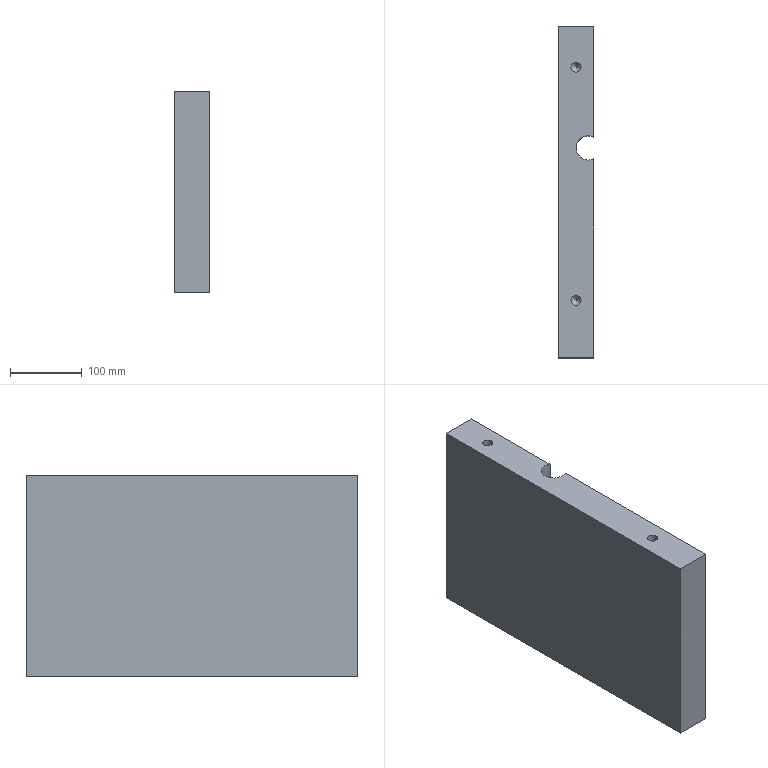Part | NX | features 29 2 | 1 solid | 16 faces | box 50 x 462.5 x 280.5 mm | volume 6261303 mm3 | plane 7 | cylinder 5 | cone 4 | commonest cylinder face diameters 14.1 x4 34 x1
STEP:
#1=CARTESIAN_POINT('',(867.05,-202.5,-493.5));
#2=VERTEX_POINT('',#1);
#3=CARTESIAN_POINT('',(860.,-202.5,-493.5));
#4=DIRECTION('',(0.,0.,1.));
#5=DIRECTION('',(1.,0.,0.));
#6=AXIS2_PLACEMENT_3D('',#3,#4,#5);
#7=CIRCLE('',#6,7.05);
#8=EDGE_CURVE('',#2,#2,#7,.T.);
#9=ORIENTED_EDGE('',*,*,#8,.T.);
#10=EDGE_LOOP('',(#9));
#11=FACE_BOUND('',#10,.T.);
#12=CARTESIAN_POINT('',(885.,-300.,-493.5));
#13=VERTEX_POINT('',#12);
#14=CARTESIAN_POINT('',(885.,-145.,-493.5));
#15=VERTEX_POINT('',#14);
#16=CARTESIAN_POINT('',(885.,193.,-493.5));
#17=DIRECTION('',(0.,1.,0.));
#18=VECTOR('',#17,1000.);
#19=LINE('',#16,#18);
#20=EDGE_CURVE('',#13,#15,#19,.T.);
#21=ORIENTED_EDGE('',*,*,#20,.F.);
#22=CARTESIAN_POINT('',(885.,-330.,-493.5));
#23=VERTEX_POINT('',#22);
#24=CARTESIAN_POINT('',(877.,-315.,-493.5));
#25=DIRECTION('',(0.,0.,1.));
#26=DIRECTION('',(-1.,0.,0.));
#27=AXIS2_PLACEMENT_3D('',#24,#25,#26);
#28=CIRCLE('',#27,17.);
#29=EDGE_CURVE('',#13,#23,#28,.T.);
#30=ORIENTED_EDGE('',*,*,#29,.T.);
#31=CARTESIAN_POINT('',(885.,-607.5,-493.5));
#32=VERTEX_POINT('',#31);
#33=CARTESIAN_POINT('',(885.,193.,-493.5));
#34=DIRECTION('',(0.,1.,0.));
#35=VECTOR('',#34,1000.);
#36=LINE('',#33,#35);
#37=EDGE_CURVE('',#32,#23,#36,.T.);
#38=ORIENTED_EDGE('',*,*,#37,.F.);
#39=CARTESIAN_POINT('',(835.,-607.5,-493.5));
#40=VERTEX_POINT('',#39);
#41=CARTESIAN_POINT('',(1635.,-607.5,-493.5));
#42=DIRECTION('',(-1.,0.,0.));
#43=VECTOR('',#42,1000.);
#44=LINE('',#41,#43);
#45=EDGE_CURVE('',#32,#40,#44,.T.);
#46=ORIENTED_EDGE('',*,*,#45,.T.);
#47=CARTESIAN_POINT('',(835.,-145.,-493.5));
#48=VERTEX_POINT('',#47);
#49=CARTESIAN_POINT('',(835.,193.,-493.5));
#50=DIRECTION('',(0.,-1.,0.));
#51=VECTOR('',#50,1000.);
#52=LINE('',#49,#51);
#53=EDGE_CURVE('',#48,#40,#52,.T.);
#54=ORIENTED_EDGE('',*,*,#53,.F.);
#55=CARTESIAN_POINT('',(1635.,-145.,-493.5));
#56=DIRECTION('',(-1.,0.,0.));
#57=VECTOR('',#56,1000.);
#58=LINE('',#55,#57);
#59=EDGE_CURVE('',#15,#48,#58,.T.);
#60=ORIENTED_EDGE('',*,*,#59,.F.);
#61=EDGE_LOOP('',(#21,#30,#38,#46,#54,#60));
#62=FACE_BOUND('',#61,.T.);
#63=CARTESIAN_POINT('',(867.05,-527.5,-493.5));
#64=VERTEX_POINT('',#63);
#65=CARTESIAN_POINT('',(860.,-527.5,-493.5));
#66=DIRECTION('',(0.,0.,1.));
#67=DIRECTION('',(1.,0.,0.));
#68=AXIS2_PLACEMENT_3D('',#65,#66,#67);
#69=CIRCLE('',#68,7.05);
#70=EDGE_CURVE('',#64,#64,#69,.T.);
#71=ORIENTED_EDGE('',*,*,#70,.T.);
#72=EDGE_LOOP('',(#71));
#73=FACE_BOUND('',#72,.T.);
#74=CARTESIAN_POINT('',(1635.,0.,-493.5));
#75=DIRECTION('',(0.,0.,-1.));
#76=DIRECTION('',(1.,0.,0.));
#77=AXIS2_PLACEMENT_3D('',#74,#75,#76);
#78=PLANE('',#77);
#79=ADVANCED_FACE('',(#11,#62,#73),#78,.T.);
#80=CARTESIAN_POINT('',(867.05,-202.5,-213.));
#81=VERTEX_POINT('',#80);
#82=CARTESIAN_POINT('',(860.,-202.5,-213.));
#83=DIRECTION('',(0.,0.,-1.));
#84=DIRECTION('',(1.,0.,0.));
#85=AXIS2_PLACEMENT_3D('',#82,#83,#84);
#86=CIRCLE('',#85,7.05);
#87=EDGE_CURVE('',#81,#81,#86,.T.);
#88=ORIENTED_EDGE('',*,*,#87,.T.);
#89=EDGE_LOOP('',(#88));
#90=FACE_BOUND('',#89,.T.);
#91=CARTESIAN_POINT('',(885.,-145.,-213.));
#92=VERTEX_POINT('',#91);
#93=CARTESIAN_POINT('',(835.,-145.,-213.));
#94=VERTEX_POINT('',#93);
#95=CARTESIAN_POINT('',(1635.,-145.,-213.));
#96=DIRECTION('',(-1.,0.,0.));
#97=VECTOR('',#96,1000.);
#98=LINE('',#95,#97);
#99=EDGE_CURVE('',#92,#94,#98,.T.);
#100=ORIENTED_EDGE('',*,*,#99,.T.);
#101=CARTESIAN_POINT('',(835.,-607.5,-213.));
#102=VERTEX_POINT('',#101);
#103=CARTESIAN_POINT('',(835.,193.,-213.));
#104=DIRECTION('',(0.,1.,0.));
#105=VECTOR('',#104,1000.);
#106=LINE('',#103,#105);
#107=EDGE_CURVE('',#102,#94,#106,.T.);
#108=ORIENTED_EDGE('',*,*,#107,.F.);
#109=CARTESIAN_POINT('',(885.,-607.5,-213.));
#110=VERTEX_POINT('',#109);
#111=CARTESIAN_POINT('',(1635.,-607.5,-213.));
#112=DIRECTION('',(1.,0.,0.));
#113=VECTOR('',#112,1000.);
#114=LINE('',#111,#113);
#115=EDGE_CURVE('',#102,#110,#114,.T.);
#116=ORIENTED_EDGE('',*,*,#115,.T.);
#117=CARTESIAN_POINT('',(885.,-330.,-213.));
#118=VERTEX_POINT('',#117);
#119=CARTESIAN_POINT('',(885.,193.,-213.));
#120=DIRECTION('',(0.,-1.,0.));
#121=VECTOR('',#120,1000.);
#122=LINE('',#119,#121);
#123=EDGE_CURVE('',#118,#110,#122,.T.);
#124=ORIENTED_EDGE('',*,*,#123,.F.);
#125=CARTESIAN_POINT('',(885.,-300.,-213.));
#126=VERTEX_POINT('',#125);
#127=CARTESIAN_POINT('',(877.,-315.,-213.));
#128=DIRECTION('',(0.,0.,-1.));
#129=DIRECTION('',(1.,0.,0.));
#130=AXIS2_PLACEMENT_3D('',#127,#128,#129);
#131=CIRCLE('',#130,17.);
#132=EDGE_CURVE('',#118,#126,#131,.T.);
#133=ORIENTED_EDGE('',*,*,#132,.T.);
#134=CARTESIAN_POINT('',(885.,193.,-213.));
#135=DIRECTION('',(0.,-1.,0.));
#136=VECTOR('',#135,1000.);
#137=LINE('',#134,#136);
#138=EDGE_CURVE('',#92,#126,#137,.T.);
#139=ORIENTED_EDGE('',*,*,#138,.F.);
#140=EDGE_LOOP('',(#100,#108,#116,#124,#133,#139));
#141=FACE_BOUND('',#140,.T.);
#142=CARTESIAN_POINT('',(867.05,-527.5,-213.));
#143=VERTEX_POINT('',#142);
#144=CARTESIAN_POINT('',(860.,-527.5,-213.));
#145=DIRECTION('',(0.,0.,-1.));
#146=DIRECTION('',(1.,0.,0.));
#147=AXIS2_PLACEMENT_3D('',#144,#145,#146);
#148=CIRCLE('',#147,7.05);
#149=EDGE_CURVE('',#143,#143,#148,.T.);
#150=ORIENTED_EDGE('',*,*,#149,.T.);
#151=EDGE_LOOP('',(#150));
#152=FACE_BOUND('',#151,.T.);
#153=CARTESIAN_POINT('',(1635.,0.,-213.));
#154=DIRECTION('',(0.,0.,1.));
#155=DIRECTION('',(-1.,0.,0.));
#156=AXIS2_PLACEMENT_3D('',#153,#154,#155);
#157=PLANE('',#156);
#158=ADVANCED_FACE('',(#90,#141,#152),#157,.T.);
#159=ORIENTED_EDGE('',*,*,#138,.T.);
#160=CARTESIAN_POINT('',(885.,-300.,-774.));
#161=DIRECTION('',(0.,0.,1.));
#162=VECTOR('',#161,1000.);
#163=LINE('',#160,#162);
#164=EDGE_CURVE('',#13,#126,#163,.T.);
#165=ORIENTED_EDGE('',*,*,#164,.F.);
#166=ORIENTED_EDGE('',*,*,#20,.T.);
#167=CARTESIAN_POINT('',(885.,-145.,-205.5));
#168=DIRECTION('',(0.,0.,-1.));
#169=VECTOR('',#168,1000.);
#170=LINE('',#167,#169);
#171=EDGE_CURVE('',#92,#15,#170,.T.);
#172=ORIENTED_EDGE('',*,*,#171,.F.);
#173=EDGE_LOOP('',(#159,#165,#166,#172));
#174=FACE_BOUND('',#173,.T.);
#175=CARTESIAN_POINT('',(885.,193.,-205.5));
#176=DIRECTION('',(1.,0.,0.));
#177=DIRECTION('',(0.,0.,-1.));
#178=AXIS2_PLACEMENT_3D('',#175,#176,#177);
#179=PLANE('',#178);
#180=ADVANCED_FACE('',(#174),#179,.T.);
#181=ORIENTED_EDGE('',*,*,#37,.T.);
#182=CARTESIAN_POINT('',(885.,-330.,-774.));
#183=DIRECTION('',(0.,0.,-1.));
#184=VECTOR('',#183,1000.);
#185=LINE('',#182,#184);
#186=EDGE_CURVE('',#118,#23,#185,.T.);
#187=ORIENTED_EDGE('',*,*,#186,.F.);
#188=ORIENTED_EDGE('',*,*,#123,.T.);
#189=CARTESIAN_POINT('',(885.,-607.5,-205.5));
#190=DIRECTION('',(0.,0.,-1.));
#191=VECTOR('',#190,1000.);
#192=LINE('',#189,#191);
#193=EDGE_CURVE('',#110,#32,#192,.T.);
#194=ORIENTED_EDGE('',*,*,#193,.T.);
#195=EDGE_LOOP('',(#181,#187,#188,#194));
#196=FACE_BOUND('',#195,.T.);
#197=CARTESIAN_POINT('',(885.,193.,-205.5));
#198=DIRECTION('',(1.,0.,0.));
#199=DIRECTION('',(0.,0.,-1.));
#200=AXIS2_PLACEMENT_3D('',#197,#198,#199);
#201=PLANE('',#200);
#202=ADVANCED_FACE('',(#196),#201,.T.);
#203=ORIENTED_EDGE('',*,*,#99,.F.);
#204=ORIENTED_EDGE('',*,*,#171,.T.);
#205=ORIENTED_EDGE('',*,*,#59,.T.);
#206=CARTESIAN_POINT('',(835.,-145.,-205.5));
#207=DIRECTION('',(0.,0.,1.));
#208=VECTOR('',#207,1000.);
#209=LINE('',#206,#208);
#210=EDGE_CURVE('',#48,#94,#209,.T.);
#211=ORIENTED_EDGE('',*,*,#210,.T.);
#212=EDGE_LOOP('',(#203,#204,#205,#211));
#213=FACE_BOUND('',#212,.T.);
#214=CARTESIAN_POINT('',(775.,-145.,-518.5));
#215=DIRECTION('',(0.,1.,0.));
#216=DIRECTION('',(0.,0.,-1.));
#217=AXIS2_PLACEMENT_3D('',#214,#215,#216);
#218=PLANE('',#217);
#219=ADVANCED_FACE('',(#213),#218,.T.);
#220=ORIENTED_EDGE('',*,*,#115,.F.);
#221=CARTESIAN_POINT('',(835.,-607.5,-205.5));
#222=DIRECTION('',(0.,0.,1.));
#223=VECTOR('',#222,1000.);
#224=LINE('',#221,#223);
#225=EDGE_CURVE('',#40,#102,#224,.T.);
#226=ORIENTED_EDGE('',*,*,#225,.F.);
#227=ORIENTED_EDGE('',*,*,#45,.F.);
#228=ORIENTED_EDGE('',*,*,#193,.F.);
#229=EDGE_LOOP('',(#220,#226,#227,#228));
#230=FACE_BOUND('',#229,.T.);
#231=CARTESIAN_POINT('',(848.,-607.5,-446.));
#232=DIRECTION('',(0.,-1.,0.));
#233=DIRECTION('',(0.,0.,1.));
#234=AXIS2_PLACEMENT_3D('',#231,#232,#233);
#235=PLANE('',#234);
#236=ADVANCED_FACE('',(#230),#235,.T.);
#237=ORIENTED_EDGE('',*,*,#107,.T.);
#238=ORIENTED_EDGE('',*,*,#210,.F.);
#239=ORIENTED_EDGE('',*,*,#53,.T.);
#240=ORIENTED_EDGE('',*,*,#225,.T.);
#241=EDGE_LOOP('',(#237,#238,#239,#240));
#242=FACE_BOUND('',#241,.T.);
#243=CARTESIAN_POINT('',(835.,193.,-205.5));
#244=DIRECTION('',(-1.,0.,0.));
#245=DIRECTION('',(0.,0.,1.));
#246=AXIS2_PLACEMENT_3D('',#243,#244,#245);
#247=PLANE('',#246);
#248=ADVANCED_FACE('',(#242),#247,.T.);
#249=ORIENTED_EDGE('',*,*,#164,.T.);
#250=ORIENTED_EDGE('',*,*,#132,.F.);
#251=ORIENTED_EDGE('',*,*,#186,.T.);
#252=ORIENTED_EDGE('',*,*,#29,.F.);
#253=EDGE_LOOP('',(#249,#250,#251,#252));
#254=FACE_BOUND('',#253,.T.);
#255=CARTESIAN_POINT('',(877.,-315.,-774.));
#256=DIRECTION('',(0.,0.,1.));
#257=DIRECTION('',(-1.,0.,0.));
#258=AXIS2_PLACEMENT_3D('',#255,#256,#257);
#259=CYLINDRICAL_SURFACE('',#258,17.);
#260=ADVANCED_FACE('',(#254),#259,.F.);
#261=CARTESIAN_POINT('',(852.95,-202.5,-249.95));
#262=VERTEX_POINT('',#261);
#263=CARTESIAN_POINT('',(860.,-202.5,-249.95));
#264=DIRECTION('',(0.,0.,-1.));
#265=DIRECTION('',(-1.,0.,0.));
#266=AXIS2_PLACEMENT_3D('',#263,#264,#265);
#267=CIRCLE('',#266,7.05);
#268=EDGE_CURVE('',#262,#262,#267,.T.);
#269=ORIENTED_EDGE('',*,*,#268,.T.);
#270=EDGE_LOOP('',(#269));
#271=FACE_BOUND('',#270,.T.);
#272=ORIENTED_EDGE('',*,*,#87,.F.);
#273=EDGE_LOOP('',(#272));
#274=FACE_BOUND('',#273,.T.);
#275=CARTESIAN_POINT('',(860.,-202.5,-213.));
#276=DIRECTION('',(0.,0.,-1.));
#277=DIRECTION('',(-1.,0.,0.));
#278=AXIS2_PLACEMENT_3D('',#275,#276,#277);
#279=CYLINDRICAL_SURFACE('',#278,7.05);
#280=ADVANCED_FACE('',(#271,#274),#279,.F.);
#281=CARTESIAN_POINT('',(860.,-202.5,-257.));
#282=VERTEX_POINT('',#281);
#283=VERTEX_LOOP('',#282);
#284=FACE_BOUND('',#283,.T.);
#285=ORIENTED_EDGE('',*,*,#268,.F.);
#286=EDGE_LOOP('',(#285));
#287=FACE_BOUND('',#286,.T.);
#288=CARTESIAN_POINT('',(860.,-202.5,-249.95));
#289=DIRECTION('',(0.,0.,1.));
#290=DIRECTION('',(-1.,0.,0.));
#291=AXIS2_PLACEMENT_3D('',#288,#289,#290);
#292=CONICAL_SURFACE('',#291,7.05,0.7854);
#293=ADVANCED_FACE('',(#284,#287),#292,.F.);
#294=CARTESIAN_POINT('',(852.95,-527.5,-249.95));
#295=VERTEX_POINT('',#294);
#296=CARTESIAN_POINT('',(860.,-527.5,-249.95));
#297=DIRECTION('',(0.,0.,-1.));
#298=DIRECTION('',(-1.,0.,0.));
#299=AXIS2_PLACEMENT_3D('',#296,#297,#298);
#300=CIRCLE('',#299,7.05);
#301=EDGE_CURVE('',#295,#295,#300,.T.);
#302=ORIENTED_EDGE('',*,*,#301,.T.);
#303=EDGE_LOOP('',(#302));
#304=FACE_BOUND('',#303,.T.);
#305=ORIENTED_EDGE('',*,*,#149,.F.);
#306=EDGE_LOOP('',(#305));
#307=FACE_BOUND('',#306,.T.);
#308=CARTESIAN_POINT('',(860.,-527.5,-213.));
#309=DIRECTION('',(0.,0.,-1.));
#310=DIRECTION('',(-1.,0.,0.));
#311=AXIS2_PLACEMENT_3D('',#308,#309,#310);
#312=CYLINDRICAL_SURFACE('',#311,7.05);
#313=ADVANCED_FACE('',(#304,#307),#312,.F.);
#314=CARTESIAN_POINT('',(860.,-527.5,-257.));
#315=VERTEX_POINT('',#314);
#316=VERTEX_LOOP('',#315);
#317=FACE_BOUND('',#316,.T.);
#318=ORIENTED_EDGE('',*,*,#301,.F.);
#319=EDGE_LOOP('',(#318));
#320=FACE_BOUND('',#319,.T.);
#321=CARTESIAN_POINT('',(860.,-527.5,-249.95));
#322=DIRECTION('',(0.,0.,1.));
#323=DIRECTION('',(-1.,0.,0.));
#324=AXIS2_PLACEMENT_3D('',#321,#322,#323);
#325=CONICAL_SURFACE('',#324,7.05,0.7854);
#326=ADVANCED_FACE('',(#317,#320),#325,.F.);
#327=CARTESIAN_POINT('',(867.05,-202.5,-456.55));
#328=VERTEX_POINT('',#327);
#329=CARTESIAN_POINT('',(860.,-202.5,-456.55));
#330=DIRECTION('',(0.,0.,1.));
#331=DIRECTION('',(1.,0.,0.));
#332=AXIS2_PLACEMENT_3D('',#329,#330,#331);
#333=CIRCLE('',#332,7.05);
#334=EDGE_CURVE('',#328,#328,#333,.T.);
#335=ORIENTED_EDGE('',*,*,#334,.T.);
#336=EDGE_LOOP('',(#335));
#337=FACE_BOUND('',#336,.T.);
#338=ORIENTED_EDGE('',*,*,#8,.F.);
#339=EDGE_LOOP('',(#338));
#340=FACE_BOUND('',#339,.T.);
#341=CARTESIAN_POINT('',(860.,-202.5,-493.5));
#342=DIRECTION('',(0.,0.,1.));
#343=DIRECTION('',(-1.,0.,0.));
#344=AXIS2_PLACEMENT_3D('',#341,#342,#343);
#345=CYLINDRICAL_SURFACE('',#344,7.05);
#346=ADVANCED_FACE('',(#337,#340),#345,.F.);
#347=CARTESIAN_POINT('',(860.,-202.5,-449.5));
#348=VERTEX_POINT('',#347);
#349=VERTEX_LOOP('',#348);
#350=FACE_BOUND('',#349,.T.);
#351=ORIENTED_EDGE('',*,*,#334,.F.);
#352=EDGE_LOOP('',(#351));
#353=FACE_BOUND('',#352,.T.);
#354=CARTESIAN_POINT('',(860.,-202.5,-456.55));
#355=DIRECTION('',(0.,0.,-1.));
#356=DIRECTION('',(1.,0.,0.));
#357=AXIS2_PLACEMENT_3D('',#354,#355,#356);
#358=CONICAL_SURFACE('',#357,7.05,0.7854);
#359=ADVANCED_FACE('',(#350,#353),#358,.F.);
#360=CARTESIAN_POINT('',(867.05,-527.5,-456.55));
#361=VERTEX_POINT('',#360);
#362=CARTESIAN_POINT('',(860.,-527.5,-456.55));
#363=DIRECTION('',(0.,0.,1.));
#364=DIRECTION('',(1.,0.,0.));
#365=AXIS2_PLACEMENT_3D('',#362,#363,#364);
#366=CIRCLE('',#365,7.05);
#367=EDGE_CURVE('',#361,#361,#366,.T.);
#368=ORIENTED_EDGE('',*,*,#367,.T.);
#369=EDGE_LOOP('',(#368));
#370=FACE_BOUND('',#369,.T.);
#371=ORIENTED_EDGE('',*,*,#70,.F.);
#372=EDGE_LOOP('',(#371));
#373=FACE_BOUND('',#372,.T.);
#374=CARTESIAN_POINT('',(860.,-527.5,-493.5));
#375=DIRECTION('',(0.,0.,1.));
#376=DIRECTION('',(-1.,0.,0.));
#377=AXIS2_PLACEMENT_3D('',#374,#375,#376);
#378=CYLINDRICAL_SURFACE('',#377,7.05);
#379=ADVANCED_FACE('',(#370,#373),#378,.F.);
#380=CARTESIAN_POINT('',(860.,-527.5,-449.5));
#381=VERTEX_POINT('',#380);
#382=VERTEX_LOOP('',#381);
#383=FACE_BOUND('',#382,.T.);
#384=ORIENTED_EDGE('',*,*,#367,.F.);
#385=EDGE_LOOP('',(#384));
#386=FACE_BOUND('',#385,.T.);
#387=CARTESIAN_POINT('',(860.,-527.5,-456.55));
#388=DIRECTION('',(0.,0.,-1.));
#389=DIRECTION('',(1.,0.,0.));
#390=AXIS2_PLACEMENT_3D('',#387,#388,#389);
#391=CONICAL_SURFACE('',#390,7.05,0.7854);
#392=ADVANCED_FACE('',(#383,#386),#391,.F.);
#393=CLOSED_SHELL('',(#79,#158,#180,#202,#219,#236,#248,#260,#280,#293,#313,#326,#346,#359,#379,#392));
#394=MANIFOLD_SOLID_BREP('',#393);
#395=(LENGTH_UNIT()NAMED_UNIT(*)SI_UNIT(.MILLI.,.METRE.));
#396=UNCERTAINTY_MEASURE_WITH_UNIT(LENGTH_MEASURE(0.00001),#395,'','');
#397=(NAMED_UNIT(*)PLANE_ANGLE_UNIT()SI_UNIT($,.RADIAN.));
#398=(NAMED_UNIT(*)SI_UNIT($,.STERADIAN.)SOLID_ANGLE_UNIT());
#399=(GEOMETRIC_REPRESENTATION_CONTEXT(3)GLOBAL_UNCERTAINTY_ASSIGNED_CONTEXT((#396))GLOBAL_UNIT_ASSIGNED_CONTEXT((#395,#397,#398))REPRESENTATION_CONTEXT('',''));
#400=ADVANCED_BREP_SHAPE_REPRESENTATION('',(#394),#399);